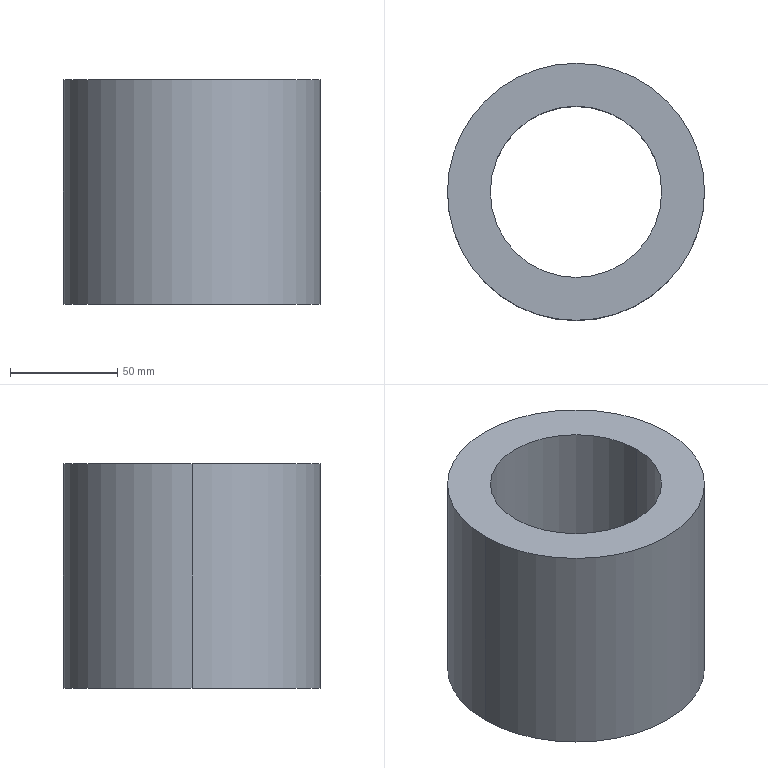Part | SolidWorks | features BaseBody 1 | 1 solid | 6 faces | box 120 x 120 x 105 mm | volume 659734 mm3 | cylinder 4 | plane 2 | commonest cylinder face diameters 80 x2 120 x2
STEP:
#1=CARTESIAN_POINT('',(-721.923,501.103,619.107));
#2=VERTEX_POINT('',#1);
#3=CARTESIAN_POINT('',(-721.923,501.103,724.107));
#4=VERTEX_POINT('',#3);
#5=CARTESIAN_POINT('',(-721.923,501.103,619.107));
#6=DIRECTION('',(0.,0.,1.));
#7=VECTOR('',#6,1000.);
#8=LINE('',#5,#7);
#9=EDGE_CURVE('',#2,#4,#8,.T.);
#10=ORIENTED_EDGE('',*,*,#9,.T.);
#11=CARTESIAN_POINT('',(-801.923,501.103,724.107));
#12=VERTEX_POINT('',#11);
#13=CARTESIAN_POINT('',(-761.923,501.103,724.107));
#14=DIRECTION('',(0.,0.,1.));
#15=DIRECTION('',(1.,0.,0.));
#16=AXIS2_PLACEMENT_3D('',#13,#14,#15);
#17=CIRCLE('',#16,40.);
#18=EDGE_CURVE('',#4,#12,#17,.T.);
#19=ORIENTED_EDGE('',*,*,#18,.T.);
#20=CARTESIAN_POINT('',(-801.923,501.103,619.107));
#21=VERTEX_POINT('',#20);
#22=CARTESIAN_POINT('',(-801.923,501.103,619.107));
#23=DIRECTION('',(0.,0.,1.));
#24=VECTOR('',#23,1000.);
#25=LINE('',#22,#24);
#26=EDGE_CURVE('',#21,#12,#25,.T.);
#27=ORIENTED_EDGE('',*,*,#26,.F.);
#28=CARTESIAN_POINT('',(-761.923,501.103,619.107));
#29=DIRECTION('',(0.,0.,1.));
#30=DIRECTION('',(1.,0.,0.));
#31=AXIS2_PLACEMENT_3D('',#28,#29,#30);
#32=CIRCLE('',#31,40.);
#33=EDGE_CURVE('',#2,#21,#32,.T.);
#34=ORIENTED_EDGE('',*,*,#33,.F.);
#35=EDGE_LOOP('',(#10,#19,#27,#34));
#36=FACE_OUTER_BOUND('',#35,.T.);
#37=CARTESIAN_POINT('',(-761.923,501.103,619.107));
#38=DIRECTION('',(0.,0.,1.));
#39=DIRECTION('',(1.,0.,0.));
#40=AXIS2_PLACEMENT_3D('',#37,#38,#39);
#41=CYLINDRICAL_SURFACE('',#40,40.);
#42=ADVANCED_FACE('',(#36),#41,.F.);
#43=CARTESIAN_POINT('',(-701.923,501.103,619.107));
#44=VERTEX_POINT('',#43);
#45=CARTESIAN_POINT('',(-701.923,501.103,724.107));
#46=VERTEX_POINT('',#45);
#47=CARTESIAN_POINT('',(-701.923,501.103,619.107));
#48=DIRECTION('',(0.,0.,1.));
#49=VECTOR('',#48,1000.);
#50=LINE('',#47,#49);
#51=EDGE_CURVE('',#44,#46,#50,.T.);
#52=ORIENTED_EDGE('',*,*,#51,.T.);
#53=CARTESIAN_POINT('',(-821.923,501.103,724.107));
#54=VERTEX_POINT('',#53);
#55=CARTESIAN_POINT('',(-761.923,501.103,724.107));
#56=DIRECTION('',(0.,0.,1.));
#57=DIRECTION('',(1.,0.,0.));
#58=AXIS2_PLACEMENT_3D('',#55,#56,#57);
#59=CIRCLE('',#58,60.);
#60=EDGE_CURVE('',#54,#46,#59,.T.);
#61=ORIENTED_EDGE('',*,*,#60,.F.);
#62=CARTESIAN_POINT('',(-821.923,501.103,619.107));
#63=VERTEX_POINT('',#62);
#64=CARTESIAN_POINT('',(-821.923,501.103,619.107));
#65=DIRECTION('',(0.,0.,1.));
#66=VECTOR('',#65,1000.);
#67=LINE('',#64,#66);
#68=EDGE_CURVE('',#63,#54,#67,.T.);
#69=ORIENTED_EDGE('',*,*,#68,.F.);
#70=CARTESIAN_POINT('',(-761.923,501.103,619.107));
#71=DIRECTION('',(0.,0.,1.));
#72=DIRECTION('',(1.,0.,0.));
#73=AXIS2_PLACEMENT_3D('',#70,#71,#72);
#74=CIRCLE('',#73,60.);
#75=EDGE_CURVE('',#63,#44,#74,.T.);
#76=ORIENTED_EDGE('',*,*,#75,.T.);
#77=EDGE_LOOP('',(#52,#61,#69,#76));
#78=FACE_OUTER_BOUND('',#77,.T.);
#79=CARTESIAN_POINT('',(-761.923,501.103,619.107));
#80=DIRECTION('',(0.,0.,1.));
#81=DIRECTION('',(1.,0.,0.));
#82=AXIS2_PLACEMENT_3D('',#79,#80,#81);
#83=CYLINDRICAL_SURFACE('',#82,60.);
#84=ADVANCED_FACE('',(#78),#83,.T.);
#85=CARTESIAN_POINT('',(-761.923,501.103,724.107));
#86=DIRECTION('',(0.,0.,1.));
#87=DIRECTION('',(1.,0.,0.));
#88=AXIS2_PLACEMENT_3D('',#85,#86,#87);
#89=CIRCLE('',#88,40.);
#90=EDGE_CURVE('',#12,#4,#89,.T.);
#91=ORIENTED_EDGE('',*,*,#90,.F.);
#92=ORIENTED_EDGE('',*,*,#18,.F.);
#93=EDGE_LOOP('',(#91,#92));
#94=FACE_BOUND('',#93,.T.);
#95=ORIENTED_EDGE('',*,*,#60,.T.);
#96=CARTESIAN_POINT('',(-761.923,501.103,724.107));
#97=DIRECTION('',(0.,0.,1.));
#98=DIRECTION('',(1.,0.,0.));
#99=AXIS2_PLACEMENT_3D('',#96,#97,#98);
#100=CIRCLE('',#99,60.);
#101=EDGE_CURVE('',#46,#54,#100,.T.);
#102=ORIENTED_EDGE('',*,*,#101,.T.);
#103=EDGE_LOOP('',(#95,#102));
#104=FACE_OUTER_BOUND('',#103,.T.);
#105=CARTESIAN_POINT('',(-761.923,501.103,724.107));
#106=DIRECTION('',(0.,0.,-1.));
#107=DIRECTION('',(0.,-1.,0.));
#108=AXIS2_PLACEMENT_3D('',#105,#106,#107);
#109=PLANE('',#108);
#110=ADVANCED_FACE('',(#94,#104),#109,.F.);
#111=CARTESIAN_POINT('',(-761.923,501.103,619.107));
#112=DIRECTION('',(0.,0.,1.));
#113=DIRECTION('',(1.,0.,0.));
#114=AXIS2_PLACEMENT_3D('',#111,#112,#113);
#115=CIRCLE('',#114,40.);
#116=EDGE_CURVE('',#21,#2,#115,.T.);
#117=ORIENTED_EDGE('',*,*,#116,.T.);
#118=ORIENTED_EDGE('',*,*,#33,.T.);
#119=EDGE_LOOP('',(#117,#118));
#120=FACE_BOUND('',#119,.T.);
#121=ORIENTED_EDGE('',*,*,#75,.F.);
#122=CARTESIAN_POINT('',(-761.923,501.103,619.107));
#123=DIRECTION('',(0.,0.,1.));
#124=DIRECTION('',(1.,0.,0.));
#125=AXIS2_PLACEMENT_3D('',#122,#123,#124);
#126=CIRCLE('',#125,60.);
#127=EDGE_CURVE('',#44,#63,#126,.T.);
#128=ORIENTED_EDGE('',*,*,#127,.F.);
#129=EDGE_LOOP('',(#121,#128));
#130=FACE_OUTER_BOUND('',#129,.T.);
#131=CARTESIAN_POINT('',(-761.923,501.103,619.107));
#132=DIRECTION('',(0.,0.,-1.));
#133=DIRECTION('',(0.,-1.,0.));
#134=AXIS2_PLACEMENT_3D('',#131,#132,#133);
#135=PLANE('',#134);
#136=ADVANCED_FACE('',(#120,#130),#135,.T.);
#137=ORIENTED_EDGE('',*,*,#127,.T.);
#138=ORIENTED_EDGE('',*,*,#68,.T.);
#139=ORIENTED_EDGE('',*,*,#101,.F.);
#140=ORIENTED_EDGE('',*,*,#51,.F.);
#141=EDGE_LOOP('',(#137,#138,#139,#140));
#142=FACE_OUTER_BOUND('',#141,.T.);
#143=CARTESIAN_POINT('',(-761.923,501.103,619.107));
#144=DIRECTION('',(0.,0.,1.));
#145=DIRECTION('',(1.,0.,0.));
#146=AXIS2_PLACEMENT_3D('',#143,#144,#145);
#147=CYLINDRICAL_SURFACE('',#146,60.);
#148=ADVANCED_FACE('',(#142),#147,.T.);
#149=ORIENTED_EDGE('',*,*,#116,.F.);
#150=ORIENTED_EDGE('',*,*,#26,.T.);
#151=ORIENTED_EDGE('',*,*,#90,.T.);
#152=ORIENTED_EDGE('',*,*,#9,.F.);
#153=EDGE_LOOP('',(#149,#150,#151,#152));
#154=FACE_OUTER_BOUND('',#153,.T.);
#155=CARTESIAN_POINT('',(-761.923,501.103,619.107));
#156=DIRECTION('',(0.,0.,1.));
#157=DIRECTION('',(1.,0.,0.));
#158=AXIS2_PLACEMENT_3D('',#155,#156,#157);
#159=CYLINDRICAL_SURFACE('',#158,40.);
#160=ADVANCED_FACE('',(#154),#159,.F.);
#161=CLOSED_SHELL('',(#42,#84,#110,#136,#148,#160));
#162=MANIFOLD_SOLID_BREP('',#161);
#163=CARTESIAN_POINT('',(0.,0.,0.));
#164=DIRECTION('',(0.,0.,1.));
#165=DIRECTION('',(1.,0.,0.));
#166=AXIS2_PLACEMENT_3D('',#163,#164,#165);
#167=(LENGTH_UNIT()NAMED_UNIT(*)SI_UNIT(.MILLI.,.METRE.));
#168=UNCERTAINTY_MEASURE_WITH_UNIT(LENGTH_MEASURE(0.00001),#167,'','');
#169=(NAMED_UNIT(*)PLANE_ANGLE_UNIT()SI_UNIT($,.RADIAN.));
#170=(NAMED_UNIT(*)SI_UNIT($,.STERADIAN.)SOLID_ANGLE_UNIT());
#171=(GEOMETRIC_REPRESENTATION_CONTEXT(3)GLOBAL_UNCERTAINTY_ASSIGNED_CONTEXT((#168))GLOBAL_UNIT_ASSIGNED_CONTEXT((#167,#169,#170))REPRESENTATION_CONTEXT('',''));
#172=ADVANCED_BREP_SHAPE_REPRESENTATION('',(#162,#166),#171);